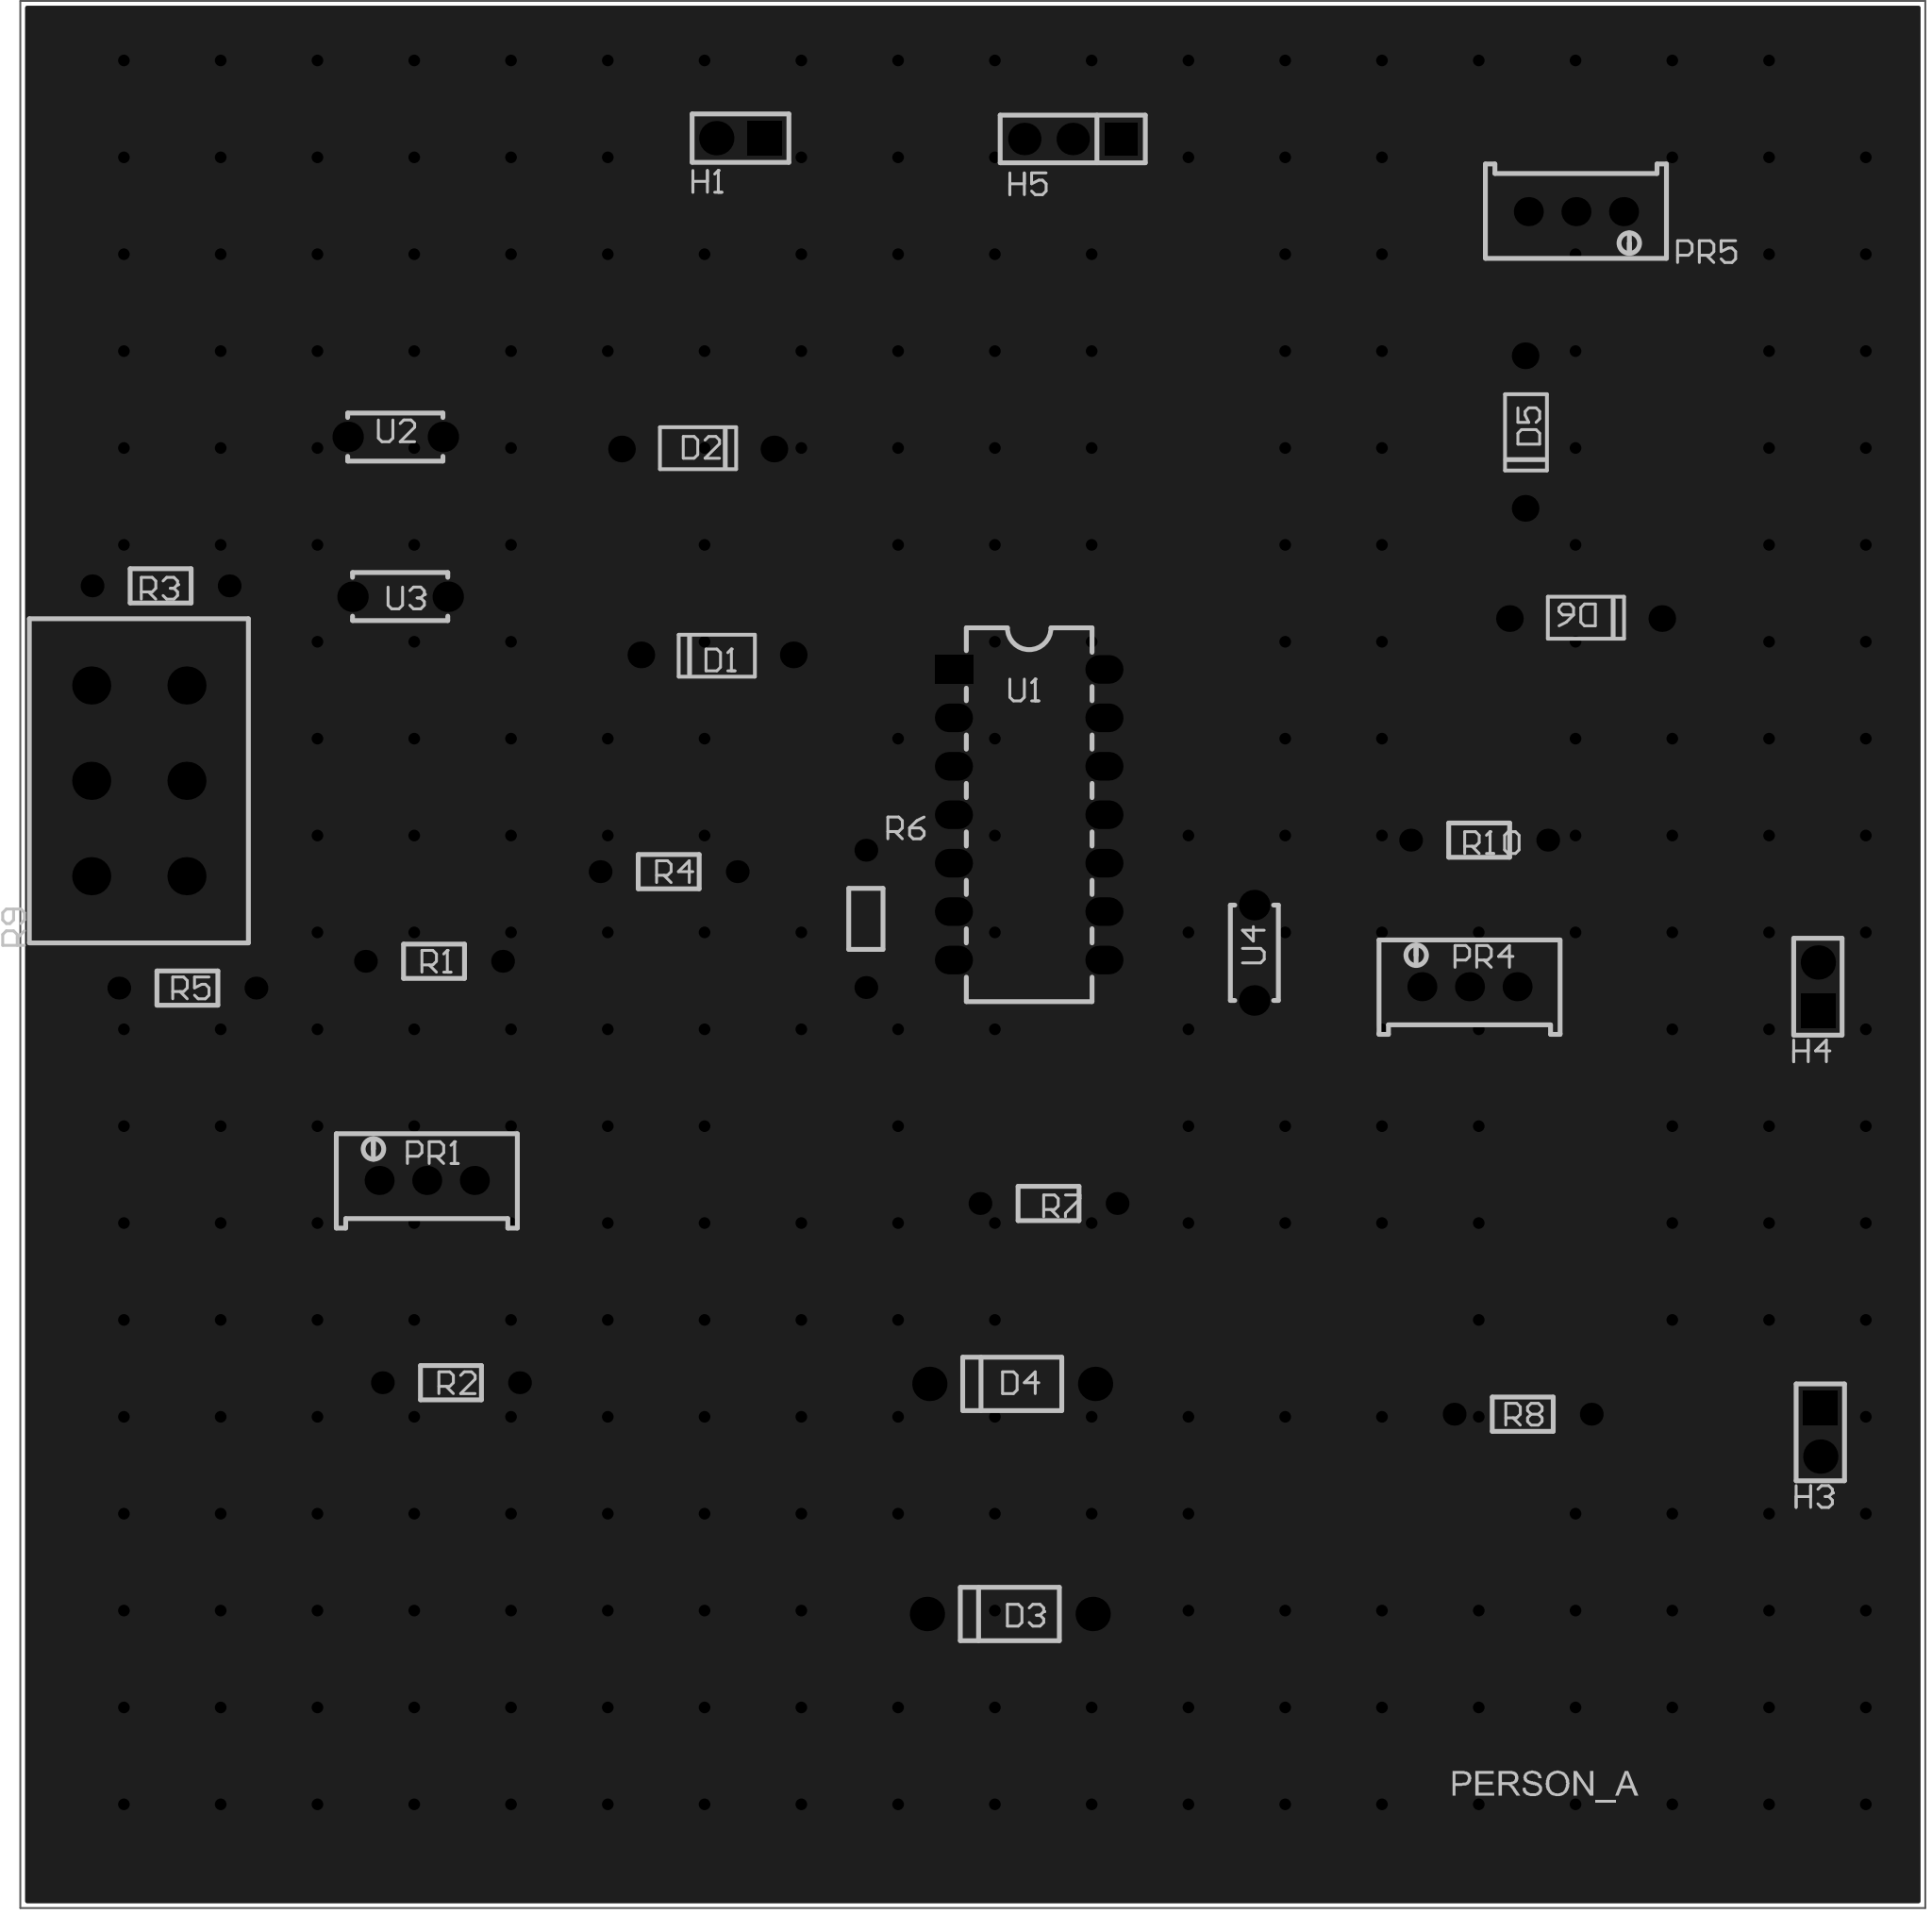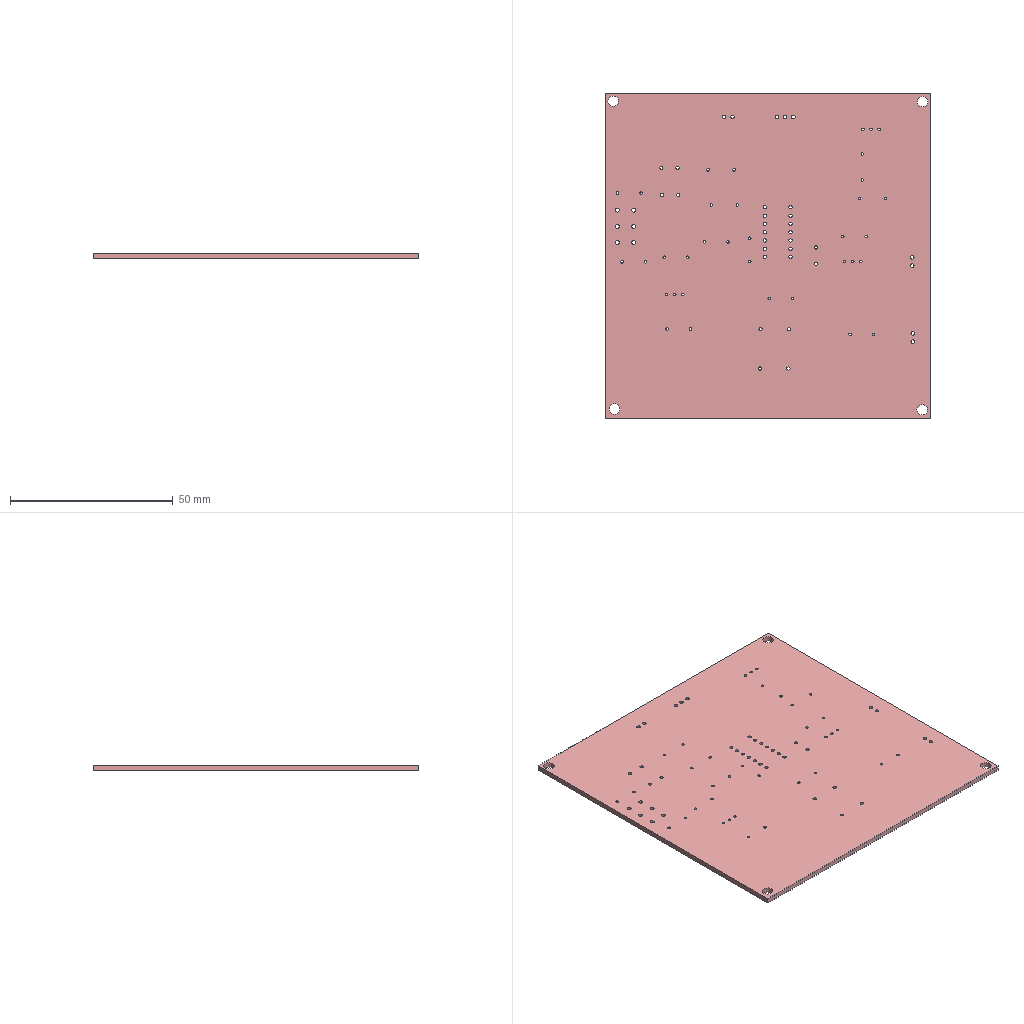Circuit board layout | Altium Designer | box 100 x 100 x 1.6 mm
Layer stack:
# Altium Designer layer stack of  (unit mm; dielectric type: 0 none, 1 core, 2 prepreg, 3 surface material)
index,name,kind,layer,copper_thickness_mm,dielectric_type,dielectric_thickness_mm,dielectric_material,dielectric_constant
0,Top Paste Mask Layer,other,,,,,,
1,Top Silkscreen Layer,other,,,,,,
2,Top Solder Mask Layer,dielectric,,,3,0.01,,3.3
3,Top Layer,copper,Top Layer,0.035,,,,
4,Dielectric1,dielectric,,,3,1.51,FR4,4.5
5,Bottom Layer,copper,Bottom Layer,0.035,,,,
6,Bottom Solder Mask Layer,dielectric,,,3,0.01,,3.3
7,Bottom Silkscreen Layer,other,,,,,,
8,Bottom Paste Mask Layer,other,,,,,,
# drill layer pairs: low layer,high layer
drill_pair,Top Layer,Bottom Layer
Part placement:
Designator,Comment,Layer,Footprint,Center-X(mm),Center-Y(mm),Rotation
D3,1N4731A,TopLayer,DO-41_BD2.4-L4.7-P8.70-D0.9-RD,130.683,100.584,0
D4,1N4731A,TopLayer,DO-41_BD2.4-L4.7-P8.70-D0.9-RD,130.81,112.649,0
H1,,TopLayer,HDR-TH_2P-P2.54-V-M-1,116.545,177.97,180
H3,,TopLayer,HDR-TH_2P-P2.54-V-M-1,173.228,110.109,270
H4,,TopLayer,HDR-TH_2P-P2.54-V-M-1,173.101,133.477,90
H5,,TopLayer,HDR-TH_3P-P2.54-V-M,133.985,177.927,180
PR1,10kΩ,TopLayer,R_3296,100.076,123.317,0
PR4,10kΩ,TopLayer,R_3296,154.813,133.477,0
R1,5.1kΩ,TopLayer,Res_1/8W,100.457,134.81,0
R2,5.1kΩ,TopLayer,Res_1/8W,101.346,112.712,0
R3,600Ω,TopLayer,Res_1/8W,86.106,154.495,0
R4,2kΩ,TopLayer,Res_1/8W,112.776,139.509,0
R5,600Ω,TopLayer,Res_1/8W,87.511,133.405,180
R6,10kΩ,TopLayer,Res_1/8W,123.126,137.033,270
R7,20kΩ,TopLayer,Res_1/8W,132.715,122.11,0
R8,100Ω,TopLayer,Res_1/8W,157.607,111.061,0
R10,10KΩ,TopLayer,Res_1/8W,155.321,141.161,180
U2,47nF,TopLayer,CAP-TH_L5.0-W2.5-P5.00-D1.0,98.425,162.306,0
U3,47nF,TopLayer,CAP-TH_L5.0-W2.5-P5.00-D1.0,98.679,153.924,180
U4,100nF,TopLayer,CAP-TH_L5.0-W2.5-P5.00-D1.0,143.51,135.255,90
U1,LF347BN/PB,TopLayer,PDIP-14_L19.6-W6.5-P2.54-LS7.9-BL,131.699,142.494,270
D1,1N4148,TopLayer,DO-35_BD2.2-L4.0-D0.50_1N4148,115.316,150.876,180
D2,1N4148,TopLayer,DO-35_BD2.2-L4.0-D0.50_1N4148,114.3,161.671,0
D5,1N4148,TopLayer,DO-35_BD2.2-L4.0-D0.50_1N4148,157.734,162.56,270
D6,1N4148,TopLayer,DO-35_BD2.2-L4.0-D0.50_1N4148,160.909,152.781,0
PR5,10kΩ,TopLayer,R_3296,160.401,174.117,180
R9,,TopLayer,WH148,84.963,144.272,90
Pad and via stacks:
# Altium Designer via and pad stacks of  (unit mm). Each distinct definition once, with the count of objects using it.
# via: kind,start_layer,end_layer,hole_mm,diameter_mm,mode(0 simple;1 top-mid-bottom;2 full stack),diameter_per_layer,count,example_net
# pad: kind,layer,hole_mm,hole_type(0 round;1 square;2 slot),plating,top_size,top_shape(1 round;2 rect;3 octagon;9 rounded rect),mid_size,bottom_size,mode,footprint,size_per_layer,count,example
pad,Multi-Layer,1,0,plated,1.8x1.8,1,1.8x1.8,1.8x1.8,0,DO-41_BD2.4-L4.7-P8.70-D0.9-RD,,4,D3.1
pad,Multi-Layer,1.1,0,plated,1.8x1.8,1,1.8x1.8,1.8x1.8,0,HDR-TH_2P-P2.54-V-M-1,,3,H1.2
pad,Multi-Layer,1.1,0,plated,1.8x1.8,2,1.8x1.8,1.8x1.8,0,HDR-TH_2P-P2.54-V-M-1,,3,H1.1
pad,Multi-Layer,1.1,0,plated,1.7x1.7,2,1.7x1.7,1.7x1.7,0,HDR-TH_3P-P2.54-V-M,,1,H5.1
pad,Multi-Layer,1.1,0,plated,1.7x1.7,1,1.7x1.7,1.7x1.7,0,HDR-TH_3P-P2.54-V-M,,2,H5.2
pad,Multi-Layer,0.762,0,plated,1.524x1.524,1,1.524x1.524,1.524x1.524,0,R_3296,,9,PR1.2
pad,Multi-Layer,0.8001,0,plated,1.199x1.199,1,1.199x1.199,1.199x1.199,0,Res_1/8W,,18,R1.1
pad,Multi-Layer,1,0,plated,1.6x1.6,1,1.6x1.6,1.6x1.6,0,CAP-TH_L5.0-W2.5-P5.00-D1.0,,6,U2.1
pad,Multi-Layer,1,0,plated,2x1.5,2,2x1.5,2x1.5,0,PDIP-14_L19.6-W6.5-P2.54-LS7.9-BL,,1,U1.1
pad,Multi-Layer,1,0,plated,2x1.5,1,2x1.5,2x1.5,0,PDIP-14_L19.6-W6.5-P2.54-LS7.9-BL,,13,U1.2
pad,Multi-Layer,0.8,0,plated,1.4x1.4,1,1.4x1.4,1.4x1.4,0,DO-35_BD2.2-L4.0-D0.50_1N4148,,8,D1.2
pad,Multi-Layer,1.2,0,plated,2x2,1,2x2,2x2,0,WH148,,6,R9.1
via,Top Layer,Bottom Layer,0.3048,0.61,0,,296,GND
Copper pours:
name,layer,net,type(0 solid;1 hatched;2 none)
Top Layer-GND,Top Layer,GND,0
Bottom Layer-GND,Bottom Layer,GND,0
Design rules, without the lines most boards share:
# Altium Designer design rules of  (exported by Altium Designer, unit mm)
# columns: name | kind | enabled | priority | scope1 | scope2 | descriptor | typed fields (field=value)
creepage | 65 | enabled | 1 | All | All | Creepage Distance Constraint =(0mil) (All),(All) |